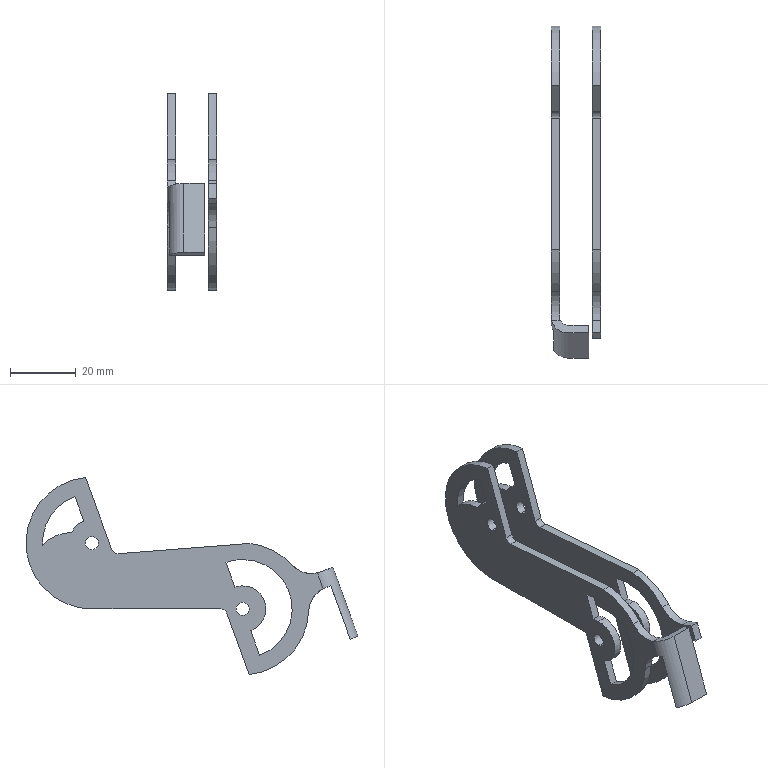Part | STEP file | Deraillieur Cage | 2 solids | 65 faces | box 15 x 100.766 x 59.814 mm | volume 9684 mm3 | cylinder 38 | plane 27 | commonest cylinder face diameters 4 x12 14 x6 30 x6 40 x6 16 x4 25 x2